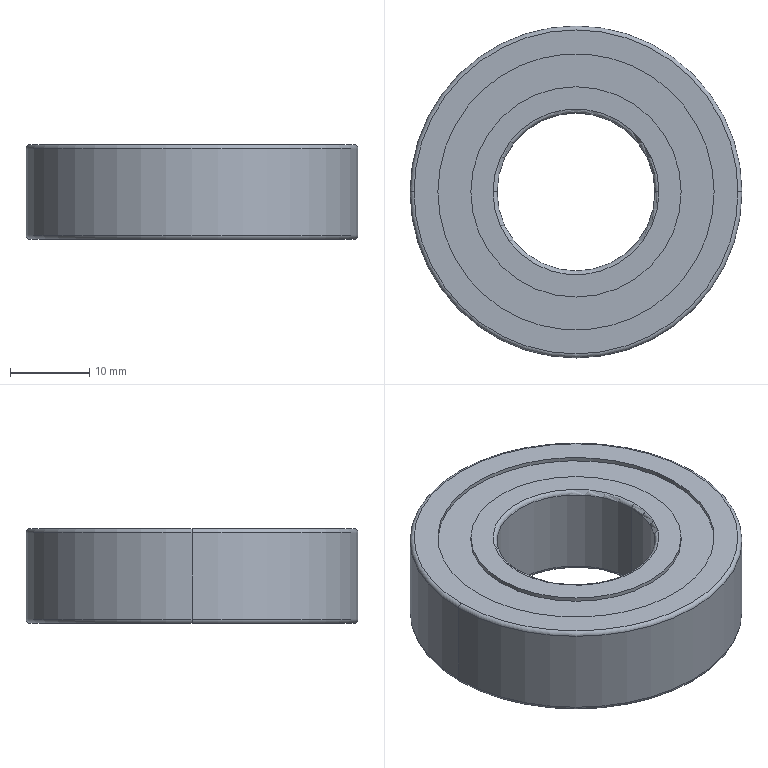Part | NX | features BREP 1 | 1 solid | 26 faces | box 42 x 42 x 12 mm | volume 12431 mm3 | cylinder 12 | torus 8 | plane 6 | commonest cylinder face diameters 26.623 x4 34.959 x4 20 x2 42 x2
STEP:
#1=CARTESIAN_POINT('',(13.311,0.,5.5));
#2=VERTEX_POINT('',#1);
#3=CARTESIAN_POINT('',(-13.311,0.,5.5));
#4=VERTEX_POINT('',#3);
#5=CARTESIAN_POINT('',(0.,0.,5.5));
#6=DIRECTION('',(0.,0.,-1.));
#7=DIRECTION('',(1.,0.,0.));
#8=AXIS2_PLACEMENT_3D('',#5,#6,#7);
#9=CIRCLE('',#8,13.311);
#10=EDGE_CURVE('',#2,#4,#9,.T.);
#11=ORIENTED_EDGE('',*,*,#10,.F.);
#12=CARTESIAN_POINT('',(13.311,0.,6.));
#13=VERTEX_POINT('',#12);
#14=CARTESIAN_POINT('',(13.311,0.,6.));
#15=DIRECTION('',(0.,0.,-1.));
#16=VECTOR('',#15,1000.);
#17=LINE('',#14,#16);
#18=EDGE_CURVE('',#13,#2,#17,.T.);
#19=ORIENTED_EDGE('',*,*,#18,.F.);
#20=CARTESIAN_POINT('',(-13.311,0.,6.));
#21=VERTEX_POINT('',#20);
#22=CARTESIAN_POINT('',(0.,0.,6.));
#23=DIRECTION('',(0.,0.,1.));
#24=DIRECTION('',(-1.,0.,0.));
#25=AXIS2_PLACEMENT_3D('',#22,#23,#24);
#26=CIRCLE('',#25,13.311);
#27=EDGE_CURVE('',#21,#13,#26,.T.);
#28=ORIENTED_EDGE('',*,*,#27,.F.);
#29=CARTESIAN_POINT('',(-13.311,0.,6.));
#30=DIRECTION('',(0.,0.,-1.));
#31=VECTOR('',#30,1000.);
#32=LINE('',#29,#31);
#33=EDGE_CURVE('',#21,#4,#32,.T.);
#34=ORIENTED_EDGE('',*,*,#33,.T.);
#35=EDGE_LOOP('',(#11,#19,#28,#34));
#36=FACE_BOUND('',#35,.T.);
#37=CARTESIAN_POINT('',(0.,0.,5.5));
#38=DIRECTION('',(0.,0.,1.));
#39=DIRECTION('',(-1.,0.,0.));
#40=AXIS2_PLACEMENT_3D('',#37,#38,#39);
#41=CYLINDRICAL_SURFACE('',#40,13.311);
#42=ADVANCED_FACE('',(#36),#41,.T.);
#43=ORIENTED_EDGE('',*,*,#33,.F.);
#44=CARTESIAN_POINT('',(0.,0.,6.));
#45=DIRECTION('',(0.,0.,1.));
#46=DIRECTION('',(1.,0.,0.));
#47=AXIS2_PLACEMENT_3D('',#44,#45,#46);
#48=CIRCLE('',#47,13.311);
#49=EDGE_CURVE('',#13,#21,#48,.T.);
#50=ORIENTED_EDGE('',*,*,#49,.F.);
#51=ORIENTED_EDGE('',*,*,#18,.T.);
#52=CARTESIAN_POINT('',(0.,0.,5.5));
#53=DIRECTION('',(0.,0.,-1.));
#54=DIRECTION('',(-1.,0.,0.));
#55=AXIS2_PLACEMENT_3D('',#52,#53,#54);
#56=CIRCLE('',#55,13.311);
#57=EDGE_CURVE('',#4,#2,#56,.T.);
#58=ORIENTED_EDGE('',*,*,#57,.F.);
#59=EDGE_LOOP('',(#43,#50,#51,#58));
#60=FACE_BOUND('',#59,.T.);
#61=CARTESIAN_POINT('',(0.,0.,5.5));
#62=DIRECTION('',(0.,0.,1.));
#63=DIRECTION('',(-1.,0.,0.));
#64=AXIS2_PLACEMENT_3D('',#61,#62,#63);
#65=CYLINDRICAL_SURFACE('',#64,13.311);
#66=ADVANCED_FACE('',(#60),#65,.T.);
#67=CARTESIAN_POINT('',(-17.479,0.,5.5));
#68=VERTEX_POINT('',#67);
#69=CARTESIAN_POINT('',(17.479,0.,5.5));
#70=VERTEX_POINT('',#69);
#71=CARTESIAN_POINT('',(0.,0.,5.5));
#72=DIRECTION('',(0.,0.,1.));
#73=DIRECTION('',(-1.,0.,0.));
#74=AXIS2_PLACEMENT_3D('',#71,#72,#73);
#75=CIRCLE('',#74,17.479);
#76=EDGE_CURVE('',#68,#70,#75,.T.);
#77=ORIENTED_EDGE('',*,*,#76,.T.);
#78=CARTESIAN_POINT('',(0.,0.,5.5));
#79=DIRECTION('',(0.,0.,1.));
#80=DIRECTION('',(1.,0.,0.));
#81=AXIS2_PLACEMENT_3D('',#78,#79,#80);
#82=CIRCLE('',#81,17.479);
#83=EDGE_CURVE('',#70,#68,#82,.T.);
#84=ORIENTED_EDGE('',*,*,#83,.T.);
#85=EDGE_LOOP('',(#77,#84));
#86=FACE_BOUND('',#85,.T.);
#87=ORIENTED_EDGE('',*,*,#10,.T.);
#88=ORIENTED_EDGE('',*,*,#57,.T.);
#89=EDGE_LOOP('',(#87,#88));
#90=FACE_BOUND('',#89,.T.);
#91=CARTESIAN_POINT('',(0.,0.,5.5));
#92=DIRECTION('',(0.,0.,1.));
#93=DIRECTION('',(-1.,0.,0.));
#94=AXIS2_PLACEMENT_3D('',#91,#92,#93);
#95=PLANE('',#94);
#96=ADVANCED_FACE('',(#86,#90),#95,.T.);
#97=ORIENTED_EDGE('',*,*,#83,.F.);
#98=CARTESIAN_POINT('',(17.479,0.,6.));
#99=VERTEX_POINT('',#98);
#100=CARTESIAN_POINT('',(17.479,0.,6.));
#101=DIRECTION('',(0.,0.,-1.));
#102=VECTOR('',#101,1000.);
#103=LINE('',#100,#102);
#104=EDGE_CURVE('',#99,#70,#103,.T.);
#105=ORIENTED_EDGE('',*,*,#104,.F.);
#106=CARTESIAN_POINT('',(-17.479,0.,6.));
#107=VERTEX_POINT('',#106);
#108=CARTESIAN_POINT('',(0.,0.,6.));
#109=DIRECTION('',(0.,0.,-1.));
#110=DIRECTION('',(-1.,0.,0.));
#111=AXIS2_PLACEMENT_3D('',#108,#109,#110);
#112=CIRCLE('',#111,17.479);
#113=EDGE_CURVE('',#107,#99,#112,.T.);
#114=ORIENTED_EDGE('',*,*,#113,.F.);
#115=CARTESIAN_POINT('',(-17.479,0.,6.));
#116=DIRECTION('',(0.,0.,-1.));
#117=VECTOR('',#116,1000.);
#118=LINE('',#115,#117);
#119=EDGE_CURVE('',#107,#68,#118,.T.);
#120=ORIENTED_EDGE('',*,*,#119,.T.);
#121=EDGE_LOOP('',(#97,#105,#114,#120));
#122=FACE_BOUND('',#121,.T.);
#123=CARTESIAN_POINT('',(0.,0.,5.5));
#124=DIRECTION('',(0.,0.,1.));
#125=DIRECTION('',(-1.,0.,0.));
#126=AXIS2_PLACEMENT_3D('',#123,#124,#125);
#127=CYLINDRICAL_SURFACE('',#126,17.479);
#128=ADVANCED_FACE('',(#122),#127,.F.);
#129=ORIENTED_EDGE('',*,*,#119,.F.);
#130=CARTESIAN_POINT('',(0.,0.,6.));
#131=DIRECTION('',(0.,0.,-1.));
#132=DIRECTION('',(1.,0.,0.));
#133=AXIS2_PLACEMENT_3D('',#130,#131,#132);
#134=CIRCLE('',#133,17.479);
#135=EDGE_CURVE('',#99,#107,#134,.T.);
#136=ORIENTED_EDGE('',*,*,#135,.F.);
#137=ORIENTED_EDGE('',*,*,#104,.T.);
#138=ORIENTED_EDGE('',*,*,#76,.F.);
#139=EDGE_LOOP('',(#129,#136,#137,#138));
#140=FACE_BOUND('',#139,.T.);
#141=CARTESIAN_POINT('',(0.,0.,5.5));
#142=DIRECTION('',(0.,0.,1.));
#143=DIRECTION('',(-1.,0.,0.));
#144=AXIS2_PLACEMENT_3D('',#141,#142,#143);
#145=CYLINDRICAL_SURFACE('',#144,17.479);
#146=ADVANCED_FACE('',(#140),#145,.F.);
#147=CARTESIAN_POINT('',(-20.5,0.,6.));
#148=VERTEX_POINT('',#147);
#149=CARTESIAN_POINT('',(20.5,0.,6.));
#150=VERTEX_POINT('',#149);
#151=CARTESIAN_POINT('',(0.,0.,6.));
#152=DIRECTION('',(0.,0.,1.));
#153=DIRECTION('',(-1.,0.,0.));
#154=AXIS2_PLACEMENT_3D('',#151,#152,#153);
#155=CIRCLE('',#154,20.5);
#156=EDGE_CURVE('',#148,#150,#155,.T.);
#157=ORIENTED_EDGE('',*,*,#156,.T.);
#158=CARTESIAN_POINT('',(0.,0.,6.));
#159=DIRECTION('',(0.,0.,1.));
#160=DIRECTION('',(1.,0.,0.));
#161=AXIS2_PLACEMENT_3D('',#158,#159,#160);
#162=CIRCLE('',#161,20.5);
#163=EDGE_CURVE('',#150,#148,#162,.T.);
#164=ORIENTED_EDGE('',*,*,#163,.T.);
#165=EDGE_LOOP('',(#157,#164));
#166=FACE_BOUND('',#165,.T.);
#167=ORIENTED_EDGE('',*,*,#135,.T.);
#168=ORIENTED_EDGE('',*,*,#113,.T.);
#169=EDGE_LOOP('',(#167,#168));
#170=FACE_BOUND('',#169,.T.);
#171=CARTESIAN_POINT('',(0.,0.,6.));
#172=DIRECTION('',(0.,0.,1.));
#173=DIRECTION('',(-1.,0.,0.));
#174=AXIS2_PLACEMENT_3D('',#171,#172,#173);
#175=PLANE('',#174);
#176=ADVANCED_FACE('',(#166,#170),#175,.T.);
#177=CARTESIAN_POINT('',(-21.,0.,5.5));
#178=VERTEX_POINT('',#177);
#179=CARTESIAN_POINT('',(-20.5,0.,5.5));
#180=DIRECTION('',(0.,-1.,0.));
#181=DIRECTION('',(0.,0.,1.));
#182=AXIS2_PLACEMENT_3D('',#179,#180,#181);
#183=CIRCLE('',#182,0.5);
#184=EDGE_CURVE('',#178,#148,#183,.F.);
#185=ORIENTED_EDGE('',*,*,#184,.T.);
#186=ORIENTED_EDGE('',*,*,#163,.F.);
#187=CARTESIAN_POINT('',(21.,0.,5.5));
#188=VERTEX_POINT('',#187);
#189=CARTESIAN_POINT('',(20.5,0.,5.5));
#190=DIRECTION('',(0.,1.,0.));
#191=DIRECTION('',(0.,0.,1.));
#192=AXIS2_PLACEMENT_3D('',#189,#190,#191);
#193=CIRCLE('',#192,0.5);
#194=EDGE_CURVE('',#188,#150,#193,.F.);
#195=ORIENTED_EDGE('',*,*,#194,.F.);
#196=CARTESIAN_POINT('',(0.,0.,5.5));
#197=DIRECTION('',(0.,0.,1.));
#198=DIRECTION('',(1.,0.,0.));
#199=AXIS2_PLACEMENT_3D('',#196,#197,#198);
#200=CIRCLE('',#199,21.);
#201=EDGE_CURVE('',#188,#178,#200,.T.);
#202=ORIENTED_EDGE('',*,*,#201,.T.);
#203=EDGE_LOOP('',(#185,#186,#195,#202));
#204=FACE_BOUND('',#203,.T.);
#205=CARTESIAN_POINT('',(0.,0.,5.5));
#206=DIRECTION('',(0.,0.,1.));
#207=DIRECTION('',(-1.,0.,0.));
#208=AXIS2_PLACEMENT_3D('',#205,#206,#207);
#209=TOROIDAL_SURFACE('',#208,20.5,0.5);
#210=ADVANCED_FACE('',(#204),#209,.T.);
#211=CARTESIAN_POINT('',(21.,0.,-5.5));
#212=VERTEX_POINT('',#211);
#213=CARTESIAN_POINT('',(21.,0.,-5.5));
#214=DIRECTION('',(0.,0.,1.));
#215=VECTOR('',#214,1000.);
#216=LINE('',#213,#215);
#217=EDGE_CURVE('',#212,#188,#216,.T.);
#218=ORIENTED_EDGE('',*,*,#217,.F.);
#219=CARTESIAN_POINT('',(-21.,0.,-5.5));
#220=VERTEX_POINT('',#219);
#221=CARTESIAN_POINT('',(0.,0.,-5.5));
#222=DIRECTION('',(0.,0.,-1.));
#223=DIRECTION('',(-1.,0.,0.));
#224=AXIS2_PLACEMENT_3D('',#221,#222,#223);
#225=CIRCLE('',#224,21.);
#226=EDGE_CURVE('',#220,#212,#225,.T.);
#227=ORIENTED_EDGE('',*,*,#226,.F.);
#228=CARTESIAN_POINT('',(-21.,0.,-5.5));
#229=DIRECTION('',(0.,0.,1.));
#230=VECTOR('',#229,1000.);
#231=LINE('',#228,#230);
#232=EDGE_CURVE('',#220,#178,#231,.T.);
#233=ORIENTED_EDGE('',*,*,#232,.T.);
#234=ORIENTED_EDGE('',*,*,#201,.F.);
#235=EDGE_LOOP('',(#218,#227,#233,#234));
#236=FACE_BOUND('',#235,.T.);
#237=CARTESIAN_POINT('',(0.,0.,6.));
#238=DIRECTION('',(0.,0.,-1.));
#239=DIRECTION('',(1.,0.,0.));
#240=AXIS2_PLACEMENT_3D('',#237,#238,#239);
#241=CYLINDRICAL_SURFACE('',#240,21.);
#242=ADVANCED_FACE('',(#236),#241,.T.);
#243=CARTESIAN_POINT('',(0.,0.,5.5));
#244=DIRECTION('',(0.,0.,1.));
#245=DIRECTION('',(-1.,0.,0.));
#246=AXIS2_PLACEMENT_3D('',#243,#244,#245);
#247=CIRCLE('',#246,21.);
#248=EDGE_CURVE('',#178,#188,#247,.T.);
#249=ORIENTED_EDGE('',*,*,#248,.F.);
#250=ORIENTED_EDGE('',*,*,#232,.F.);
#251=CARTESIAN_POINT('',(0.,0.,-5.5));
#252=DIRECTION('',(0.,0.,-1.));
#253=DIRECTION('',(1.,0.,0.));
#254=AXIS2_PLACEMENT_3D('',#251,#252,#253);
#255=CIRCLE('',#254,21.);
#256=EDGE_CURVE('',#212,#220,#255,.T.);
#257=ORIENTED_EDGE('',*,*,#256,.F.);
#258=ORIENTED_EDGE('',*,*,#217,.T.);
#259=EDGE_LOOP('',(#249,#250,#257,#258));
#260=FACE_BOUND('',#259,.T.);
#261=CARTESIAN_POINT('',(0.,0.,6.));
#262=DIRECTION('',(0.,0.,-1.));
#263=DIRECTION('',(1.,0.,0.));
#264=AXIS2_PLACEMENT_3D('',#261,#262,#263);
#265=CYLINDRICAL_SURFACE('',#264,21.);
#266=ADVANCED_FACE('',(#260),#265,.T.);
#267=CARTESIAN_POINT('',(20.5,0.,-6.));
#268=VERTEX_POINT('',#267);
#269=CARTESIAN_POINT('',(-20.5,0.,-6.));
#270=VERTEX_POINT('',#269);
#271=CARTESIAN_POINT('',(0.,0.,-6.));
#272=DIRECTION('',(0.,0.,-1.));
#273=DIRECTION('',(1.,0.,0.));
#274=AXIS2_PLACEMENT_3D('',#271,#272,#273);
#275=CIRCLE('',#274,20.5);
#276=EDGE_CURVE('',#268,#270,#275,.T.);
#277=ORIENTED_EDGE('',*,*,#276,.F.);
#278=CARTESIAN_POINT('',(20.5,0.,-5.5));
#279=DIRECTION('',(0.,1.,0.));
#280=DIRECTION('',(1.,0.,0.));
#281=AXIS2_PLACEMENT_3D('',#278,#279,#280);
#282=CIRCLE('',#281,0.5);
#283=EDGE_CURVE('',#212,#268,#282,.T.);
#284=ORIENTED_EDGE('',*,*,#283,.F.);
#285=ORIENTED_EDGE('',*,*,#256,.T.);
#286=CARTESIAN_POINT('',(-20.5,0.,-5.5));
#287=DIRECTION('',(0.,-1.,0.));
#288=DIRECTION('',(-1.,0.,0.));
#289=AXIS2_PLACEMENT_3D('',#286,#287,#288);
#290=CIRCLE('',#289,0.5);
#291=EDGE_CURVE('',#220,#270,#290,.T.);
#292=ORIENTED_EDGE('',*,*,#291,.T.);
#293=EDGE_LOOP('',(#277,#284,#285,#292));
#294=FACE_BOUND('',#293,.T.);
#295=CARTESIAN_POINT('',(0.,0.,-5.5));
#296=DIRECTION('',(0.,0.,1.));
#297=DIRECTION('',(-1.,0.,0.));
#298=AXIS2_PLACEMENT_3D('',#295,#296,#297);
#299=TOROIDAL_SURFACE('',#298,20.5,0.5);
#300=ADVANCED_FACE('',(#294),#299,.T.);
#301=ORIENTED_EDGE('',*,*,#291,.F.);
#302=ORIENTED_EDGE('',*,*,#226,.T.);
#303=ORIENTED_EDGE('',*,*,#283,.T.);
#304=CARTESIAN_POINT('',(0.,0.,-6.));
#305=DIRECTION('',(0.,0.,-1.));
#306=DIRECTION('',(-1.,0.,0.));
#307=AXIS2_PLACEMENT_3D('',#304,#305,#306);
#308=CIRCLE('',#307,20.5);
#309=EDGE_CURVE('',#270,#268,#308,.T.);
#310=ORIENTED_EDGE('',*,*,#309,.F.);
#311=EDGE_LOOP('',(#301,#302,#303,#310));
#312=FACE_BOUND('',#311,.T.);
#313=CARTESIAN_POINT('',(0.,0.,-5.5));
#314=DIRECTION('',(0.,0.,1.));
#315=DIRECTION('',(-1.,0.,0.));
#316=AXIS2_PLACEMENT_3D('',#313,#314,#315);
#317=TOROIDAL_SURFACE('',#316,20.5,0.5);
#318=ADVANCED_FACE('',(#312),#317,.T.);
#319=ORIENTED_EDGE('',*,*,#309,.T.);
#320=ORIENTED_EDGE('',*,*,#276,.T.);
#321=EDGE_LOOP('',(#319,#320));
#322=FACE_BOUND('',#321,.T.);
#323=CARTESIAN_POINT('',(17.479,0.,-6.));
#324=VERTEX_POINT('',#323);
#325=CARTESIAN_POINT('',(-17.479,0.,-6.));
#326=VERTEX_POINT('',#325);
#327=CARTESIAN_POINT('',(0.,0.,-6.));
#328=DIRECTION('',(0.,0.,1.));
#329=DIRECTION('',(1.,0.,0.));
#330=AXIS2_PLACEMENT_3D('',#327,#328,#329);
#331=CIRCLE('',#330,17.479);
#332=EDGE_CURVE('',#324,#326,#331,.T.);
#333=ORIENTED_EDGE('',*,*,#332,.T.);
#334=CARTESIAN_POINT('',(0.,0.,-6.));
#335=DIRECTION('',(0.,0.,1.));
#336=DIRECTION('',(-1.,0.,0.));
#337=AXIS2_PLACEMENT_3D('',#334,#335,#336);
#338=CIRCLE('',#337,17.479);
#339=EDGE_CURVE('',#326,#324,#338,.T.);
#340=ORIENTED_EDGE('',*,*,#339,.T.);
#341=EDGE_LOOP('',(#333,#340));
#342=FACE_BOUND('',#341,.T.);
#343=CARTESIAN_POINT('',(0.,0.,-6.));
#344=DIRECTION('',(0.,0.,1.));
#345=DIRECTION('',(-1.,0.,0.));
#346=AXIS2_PLACEMENT_3D('',#343,#344,#345);
#347=PLANE('',#346);
#348=ADVANCED_FACE('',(#322,#342),#347,.F.);
#349=CARTESIAN_POINT('',(17.479,0.,-5.5));
#350=VERTEX_POINT('',#349);
#351=CARTESIAN_POINT('',(17.479,0.,-6.));
#352=DIRECTION('',(0.,0.,1.));
#353=VECTOR('',#352,1000.);
#354=LINE('',#351,#353);
#355=EDGE_CURVE('',#324,#350,#354,.T.);
#356=ORIENTED_EDGE('',*,*,#355,.F.);
#357=ORIENTED_EDGE('',*,*,#339,.F.);
#358=CARTESIAN_POINT('',(-17.479,0.,-5.5));
#359=VERTEX_POINT('',#358);
#360=CARTESIAN_POINT('',(-17.479,0.,-6.));
#361=DIRECTION('',(0.,0.,1.));
#362=VECTOR('',#361,1000.);
#363=LINE('',#360,#362);
#364=EDGE_CURVE('',#326,#359,#363,.T.);
#365=ORIENTED_EDGE('',*,*,#364,.T.);
#366=CARTESIAN_POINT('',(0.,0.,-5.5));
#367=DIRECTION('',(0.,0.,-1.));
#368=DIRECTION('',(1.,0.,0.));
#369=AXIS2_PLACEMENT_3D('',#366,#367,#368);
#370=CIRCLE('',#369,17.479);
#371=EDGE_CURVE('',#350,#359,#370,.T.);
#372=ORIENTED_EDGE('',*,*,#371,.F.);
#373=EDGE_LOOP('',(#356,#357,#365,#372));
#374=FACE_BOUND('',#373,.T.);
#375=CARTESIAN_POINT('',(0.,0.,-5.5));
#376=DIRECTION('',(0.,0.,-1.));
#377=DIRECTION('',(1.,0.,0.));
#378=AXIS2_PLACEMENT_3D('',#375,#376,#377);
#379=CYLINDRICAL_SURFACE('',#378,17.479);
#380=ADVANCED_FACE('',(#374),#379,.F.);
#381=CARTESIAN_POINT('',(0.,0.,-5.5));
#382=DIRECTION('',(0.,0.,-1.));
#383=DIRECTION('',(-1.,0.,0.));
#384=AXIS2_PLACEMENT_3D('',#381,#382,#383);
#385=CIRCLE('',#384,17.479);
#386=EDGE_CURVE('',#359,#350,#385,.T.);
#387=ORIENTED_EDGE('',*,*,#386,.T.);
#388=ORIENTED_EDGE('',*,*,#371,.T.);
#389=EDGE_LOOP('',(#387,#388));
#390=FACE_BOUND('',#389,.T.);
#391=CARTESIAN_POINT('',(13.311,0.,-5.5));
#392=VERTEX_POINT('',#391);
#393=CARTESIAN_POINT('',(-13.311,0.,-5.5));
#394=VERTEX_POINT('',#393);
#395=CARTESIAN_POINT('',(0.,0.,-5.5));
#396=DIRECTION('',(0.,0.,1.));
#397=DIRECTION('',(1.,0.,0.));
#398=AXIS2_PLACEMENT_3D('',#395,#396,#397);
#399=CIRCLE('',#398,13.311);
#400=EDGE_CURVE('',#392,#394,#399,.T.);
#401=ORIENTED_EDGE('',*,*,#400,.T.);
#402=CARTESIAN_POINT('',(0.,0.,-5.5));
#403=DIRECTION('',(0.,0.,1.));
#404=DIRECTION('',(-1.,0.,0.));
#405=AXIS2_PLACEMENT_3D('',#402,#403,#404);
#406=CIRCLE('',#405,13.311);
#407=EDGE_CURVE('',#394,#392,#406,.T.);
#408=ORIENTED_EDGE('',*,*,#407,.T.);
#409=EDGE_LOOP('',(#401,#408));
#410=FACE_BOUND('',#409,.T.);
#411=CARTESIAN_POINT('',(0.,0.,-5.5));
#412=DIRECTION('',(0.,0.,-1.));
#413=DIRECTION('',(-1.,0.,0.));
#414=AXIS2_PLACEMENT_3D('',#411,#412,#413);
#415=PLANE('',#414);
#416=ADVANCED_FACE('',(#390,#410),#415,.T.);
#417=ORIENTED_EDGE('',*,*,#386,.F.);
#418=ORIENTED_EDGE('',*,*,#364,.F.);
#419=ORIENTED_EDGE('',*,*,#332,.F.);
#420=ORIENTED_EDGE('',*,*,#355,.T.);
#421=EDGE_LOOP('',(#417,#418,#419,#420));
#422=FACE_BOUND('',#421,.T.);
#423=CARTESIAN_POINT('',(0.,0.,-5.5));
#424=DIRECTION('',(0.,0.,-1.));
#425=DIRECTION('',(1.,0.,0.));
#426=AXIS2_PLACEMENT_3D('',#423,#424,#425);
#427=CYLINDRICAL_SURFACE('',#426,17.479);
#428=ADVANCED_FACE('',(#422),#427,.F.);
#429=ORIENTED_EDGE('',*,*,#407,.F.);
#430=CARTESIAN_POINT('',(-13.311,0.,-6.));
#431=VERTEX_POINT('',#430);
#432=CARTESIAN_POINT('',(-13.311,0.,-6.));
#433=DIRECTION('',(0.,0.,1.));
#434=VECTOR('',#433,1000.);
#435=LINE('',#432,#434);
#436=EDGE_CURVE('',#394,#431,#435,.F.);
#437=ORIENTED_EDGE('',*,*,#436,.T.);
#438=CARTESIAN_POINT('',(13.311,0.,-6.));
#439=VERTEX_POINT('',#438);
#440=CARTESIAN_POINT('',(0.,0.,-6.));
#441=DIRECTION('',(0.,0.,-1.));
#442=DIRECTION('',(1.,0.,0.));
#443=AXIS2_PLACEMENT_3D('',#440,#441,#442);
#444=CIRCLE('',#443,13.311);
#445=EDGE_CURVE('',#439,#431,#444,.T.);
#446=ORIENTED_EDGE('',*,*,#445,.F.);
#447=CARTESIAN_POINT('',(13.311,0.,-6.));
#448=DIRECTION('',(0.,0.,1.));
#449=VECTOR('',#448,1000.);
#450=LINE('',#447,#449);
#451=EDGE_CURVE('',#392,#439,#450,.F.);
#452=ORIENTED_EDGE('',*,*,#451,.F.);
#453=EDGE_LOOP('',(#429,#437,#446,#452));
#454=FACE_BOUND('',#453,.T.);
#455=CARTESIAN_POINT('',(0.,0.,-5.5));
#456=DIRECTION('',(0.,0.,-1.));
#457=DIRECTION('',(1.,0.,0.));
#458=AXIS2_PLACEMENT_3D('',#455,#456,#457);
#459=CYLINDRICAL_SURFACE('',#458,13.311);
#460=ADVANCED_FACE('',(#454),#459,.T.);
#461=ORIENTED_EDGE('',*,*,#451,.T.);
#462=CARTESIAN_POINT('',(0.,0.,-6.));
#463=DIRECTION('',(0.,0.,-1.));
#464=DIRECTION('',(-1.,0.,0.));
#465=AXIS2_PLACEMENT_3D('',#462,#463,#464);
#466=CIRCLE('',#465,13.311);
#467=EDGE_CURVE('',#431,#439,#466,.T.);
#468=ORIENTED_EDGE('',*,*,#467,.F.);
#469=ORIENTED_EDGE('',*,*,#436,.F.);
#470=ORIENTED_EDGE('',*,*,#400,.F.);
#471=EDGE_LOOP('',(#461,#468,#469,#470));
#472=FACE_BOUND('',#471,.T.);
#473=CARTESIAN_POINT('',(0.,0.,-5.5));
#474=DIRECTION('',(0.,0.,-1.));
#475=DIRECTION('',(1.,0.,0.));
#476=AXIS2_PLACEMENT_3D('',#473,#474,#475);
#477=CYLINDRICAL_SURFACE('',#476,13.311);
#478=ADVANCED_FACE('',(#472),#477,.T.);
#479=ORIENTED_EDGE('',*,*,#467,.T.);
#480=ORIENTED_EDGE('',*,*,#445,.T.);
#481=EDGE_LOOP('',(#479,#480));
#482=FACE_BOUND('',#481,.T.);
#483=CARTESIAN_POINT('',(-10.5,0.,-6.));
#484=VERTEX_POINT('',#483);
#485=CARTESIAN_POINT('',(10.5,0.,-6.));
#486=VERTEX_POINT('',#485);
#487=CARTESIAN_POINT('',(0.,0.,-6.));
#488=DIRECTION('',(0.,0.,1.));
#489=DIRECTION('',(-1.,0.,0.));
#490=AXIS2_PLACEMENT_3D('',#487,#488,#489);
#491=CIRCLE('',#490,10.5);
#492=EDGE_CURVE('',#484,#486,#491,.T.);
#493=ORIENTED_EDGE('',*,*,#492,.T.);
#494=CARTESIAN_POINT('',(0.,0.,-6.));
#495=DIRECTION('',(0.,0.,1.));
#496=DIRECTION('',(1.,0.,0.));
#497=AXIS2_PLACEMENT_3D('',#494,#495,#496);
#498=CIRCLE('',#497,10.5);
#499=EDGE_CURVE('',#486,#484,#498,.T.);
#500=ORIENTED_EDGE('',*,*,#499,.T.);
#501=EDGE_LOOP('',(#493,#500));
#502=FACE_BOUND('',#501,.T.);
#503=CARTESIAN_POINT('',(0.,0.,-6.));
#504=DIRECTION('',(0.,0.,1.));
#505=DIRECTION('',(-1.,0.,0.));
#506=AXIS2_PLACEMENT_3D('',#503,#504,#505);
#507=PLANE('',#506);
#508=ADVANCED_FACE('',(#482,#502),#507,.F.);
#509=CARTESIAN_POINT('',(-10.,0.,-5.5));
#510=VERTEX_POINT('',#509);
#511=CARTESIAN_POINT('',(-10.5,0.,-5.5));
#512=DIRECTION('',(0.,-1.,0.));
#513=DIRECTION('',(0.,0.,-1.));
#514=AXIS2_PLACEMENT_3D('',#511,#512,#513);
#515=CIRCLE('',#514,0.5);
#516=EDGE_CURVE('',#510,#484,#515,.F.);
#517=ORIENTED_EDGE('',*,*,#516,.T.);
#518=ORIENTED_EDGE('',*,*,#499,.F.);
#519=CARTESIAN_POINT('',(10.,0.,-5.5));
#520=VERTEX_POINT('',#519);
#521=CARTESIAN_POINT('',(10.5,0.,-5.5));
#522=DIRECTION('',(0.,1.,0.));
#523=DIRECTION('',(0.,0.,-1.));
#524=AXIS2_PLACEMENT_3D('',#521,#522,#523);
#525=CIRCLE('',#524,0.5);
#526=EDGE_CURVE('',#520,#486,#525,.F.);
#527=ORIENTED_EDGE('',*,*,#526,.F.);
#528=CARTESIAN_POINT('',(0.,0.,-5.5));
#529=DIRECTION('',(0.,0.,1.));
#530=DIRECTION('',(1.,0.,0.));
#531=AXIS2_PLACEMENT_3D('',#528,#529,#530);
#532=CIRCLE('',#531,10.);
#533=EDGE_CURVE('',#520,#510,#532,.T.);
#534=ORIENTED_EDGE('',*,*,#533,.T.);
#535=EDGE_LOOP('',(#517,#518,#527,#534));
#536=FACE_BOUND('',#535,.T.);
#537=CARTESIAN_POINT('',(0.,0.,-5.5));
#538=DIRECTION('',(0.,0.,1.));
#539=DIRECTION('',(-1.,0.,0.));
#540=AXIS2_PLACEMENT_3D('',#537,#538,#539);
#541=TOROIDAL_SURFACE('',#540,10.5,0.5);
#542=ADVANCED_FACE('',(#536),#541,.T.);
#543=CARTESIAN_POINT('',(-10.,0.,5.5));
#544=VERTEX_POINT('',#543);
#545=CARTESIAN_POINT('',(10.,0.,5.5));
#546=VERTEX_POINT('',#545);
#547=CARTESIAN_POINT('',(0.,0.,5.5));
#548=DIRECTION('',(0.,0.,-1.));
#549=DIRECTION('',(-1.,0.,0.));
#550=AXIS2_PLACEMENT_3D('',#547,#548,#549);
#551=CIRCLE('',#550,10.);
#552=EDGE_CURVE('',#544,#546,#551,.T.);
#553=ORIENTED_EDGE('',*,*,#552,.F.);
#554=CARTESIAN_POINT('',(-10.,0.,-5.5));
#555=DIRECTION('',(0.,0.,1.));
#556=VECTOR('',#555,1000.);
#557=LINE('',#554,#556);
#558=EDGE_CURVE('',#544,#510,#557,.F.);
#559=ORIENTED_EDGE('',*,*,#558,.T.);
#560=ORIENTED_EDGE('',*,*,#533,.F.);
#561=CARTESIAN_POINT('',(10.,0.,-5.5));
#562=DIRECTION('',(0.,0.,1.));
#563=VECTOR('',#562,1000.);
#564=LINE('',#561,#563);
#565=EDGE_CURVE('',#546,#520,#564,.F.);
#566=ORIENTED_EDGE('',*,*,#565,.F.);
#567=EDGE_LOOP('',(#553,#559,#560,#566));
#568=FACE_BOUND('',#567,.T.);
#569=CARTESIAN_POINT('',(0.,0.,6.));
#570=DIRECTION('',(0.,0.,-1.));
#571=DIRECTION('',(1.,0.,0.));
#572=AXIS2_PLACEMENT_3D('',#569,#570,#571);
#573=CYLINDRICAL_SURFACE('',#572,10.);
#574=ADVANCED_FACE('',(#568),#573,.F.);
#575=ORIENTED_EDGE('',*,*,#565,.T.);
#576=CARTESIAN_POINT('',(0.,0.,-5.5));
#577=DIRECTION('',(0.,0.,1.));
#578=DIRECTION('',(-1.,0.,0.));
#579=AXIS2_PLACEMENT_3D('',#576,#577,#578);
#580=CIRCLE('',#579,10.);
#581=EDGE_CURVE('',#510,#520,#580,.T.);
#582=ORIENTED_EDGE('',*,*,#581,.F.);
#583=ORIENTED_EDGE('',*,*,#558,.F.);
#584=CARTESIAN_POINT('',(0.,0.,5.5));
#585=DIRECTION('',(0.,0.,-1.));
#586=DIRECTION('',(1.,0.,0.));
#587=AXIS2_PLACEMENT_3D('',#584,#585,#586);
#588=CIRCLE('',#587,10.);
#589=EDGE_CURVE('',#546,#544,#588,.T.);
#590=ORIENTED_EDGE('',*,*,#589,.F.);
#591=EDGE_LOOP('',(#575,#582,#583,#590));
#592=FACE_BOUND('',#591,.T.);
#593=CARTESIAN_POINT('',(0.,0.,6.));
#594=DIRECTION('',(0.,0.,-1.));
#595=DIRECTION('',(1.,0.,0.));
#596=AXIS2_PLACEMENT_3D('',#593,#594,#595);
#597=CYLINDRICAL_SURFACE('',#596,10.);
#598=ADVANCED_FACE('',(#592),#597,.F.);
#599=CARTESIAN_POINT('',(10.5,0.,6.));
#600=VERTEX_POINT('',#599);
#601=CARTESIAN_POINT('',(-10.5,0.,6.));
#602=VERTEX_POINT('',#601);
#603=CARTESIAN_POINT('',(0.,0.,6.));
#604=DIRECTION('',(0.,0.,-1.));
#605=DIRECTION('',(1.,0.,0.));
#606=AXIS2_PLACEMENT_3D('',#603,#604,#605);
#607=CIRCLE('',#606,10.5);
#608=EDGE_CURVE('',#600,#602,#607,.T.);
#609=ORIENTED_EDGE('',*,*,#608,.F.);
#610=CARTESIAN_POINT('',(10.5,0.,5.5));
#611=DIRECTION('',(0.,1.,0.));
#612=DIRECTION('',(-1.,0.,0.));
#613=AXIS2_PLACEMENT_3D('',#610,#611,#612);
#614=CIRCLE('',#613,0.5);
#615=EDGE_CURVE('',#546,#600,#614,.T.);
#616=ORIENTED_EDGE('',*,*,#615,.F.);
#617=ORIENTED_EDGE('',*,*,#589,.T.);
#618=CARTESIAN_POINT('',(-10.5,0.,5.5));
#619=DIRECTION('',(0.,-1.,0.));
#620=DIRECTION('',(1.,0.,0.));
#621=AXIS2_PLACEMENT_3D('',#618,#619,#620);
#622=CIRCLE('',#621,0.5);
#623=EDGE_CURVE('',#544,#602,#622,.T.);
#624=ORIENTED_EDGE('',*,*,#623,.T.);
#625=EDGE_LOOP('',(#609,#616,#617,#624));
#626=FACE_BOUND('',#625,.T.);
#627=CARTESIAN_POINT('',(0.,0.,5.5));
#628=DIRECTION('',(0.,0.,1.));
#629=DIRECTION('',(-1.,0.,0.));
#630=AXIS2_PLACEMENT_3D('',#627,#628,#629);
#631=TOROIDAL_SURFACE('',#630,10.5,0.5);
#632=ADVANCED_FACE('',(#626),#631,.T.);
#633=ORIENTED_EDGE('',*,*,#623,.F.);
#634=ORIENTED_EDGE('',*,*,#552,.T.);
#635=ORIENTED_EDGE('',*,*,#615,.T.);
#636=CARTESIAN_POINT('',(0.,0.,6.));
#637=DIRECTION('',(0.,0.,-1.));
#638=DIRECTION('',(-1.,0.,0.));
#639=AXIS2_PLACEMENT_3D('',#636,#637,#638);
#640=CIRCLE('',#639,10.5);
#641=EDGE_CURVE('',#602,#600,#640,.T.);
#642=ORIENTED_EDGE('',*,*,#641,.F.);
#643=EDGE_LOOP('',(#633,#634,#635,#642));
#644=FACE_BOUND('',#643,.T.);
#645=CARTESIAN_POINT('',(0.,0.,5.5));
#646=DIRECTION('',(0.,0.,1.));
#647=DIRECTION('',(-1.,0.,0.));
#648=AXIS2_PLACEMENT_3D('',#645,#646,#647);
#649=TOROIDAL_SURFACE('',#648,10.5,0.5);
#650=ADVANCED_FACE('',(#644),#649,.T.);
#651=ORIENTED_EDGE('',*,*,#27,.T.);
#652=ORIENTED_EDGE('',*,*,#49,.T.);
#653=EDGE_LOOP('',(#651,#652));
#654=FACE_BOUND('',#653,.T.);
#655=ORIENTED_EDGE('',*,*,#641,.T.);
#656=ORIENTED_EDGE('',*,*,#608,.T.);
#657=EDGE_LOOP('',(#655,#656));
#658=FACE_BOUND('',#657,.T.);
#659=CARTESIAN_POINT('',(0.,0.,6.));
#660=DIRECTION('',(0.,0.,1.));
#661=DIRECTION('',(-1.,0.,0.));
#662=AXIS2_PLACEMENT_3D('',#659,#660,#661);
#663=PLANE('',#662);
#664=ADVANCED_FACE('',(#654,#658),#663,.T.);
#665=ORIENTED_EDGE('',*,*,#581,.T.);
#666=ORIENTED_EDGE('',*,*,#526,.T.);
#667=ORIENTED_EDGE('',*,*,#492,.F.);
#668=ORIENTED_EDGE('',*,*,#516,.F.);
#669=EDGE_LOOP('',(#665,#666,#667,#668));
#670=FACE_BOUND('',#669,.T.);
#671=CARTESIAN_POINT('',(0.,0.,-5.5));
#672=DIRECTION('',(0.,0.,1.));
#673=DIRECTION('',(-1.,0.,0.));
#674=AXIS2_PLACEMENT_3D('',#671,#672,#673);
#675=TOROIDAL_SURFACE('',#674,10.5,0.5);
#676=ADVANCED_FACE('',(#670),#675,.T.);
#677=ORIENTED_EDGE('',*,*,#248,.T.);
#678=ORIENTED_EDGE('',*,*,#194,.T.);
#679=ORIENTED_EDGE('',*,*,#156,.F.);
#680=ORIENTED_EDGE('',*,*,#184,.F.);
#681=EDGE_LOOP('',(#677,#678,#679,#680));
#682=FACE_BOUND('',#681,.T.);
#683=CARTESIAN_POINT('',(0.,0.,5.5));
#684=DIRECTION('',(0.,0.,1.));
#685=DIRECTION('',(-1.,0.,0.));
#686=AXIS2_PLACEMENT_3D('',#683,#684,#685);
#687=TOROIDAL_SURFACE('',#686,20.5,0.5);
#688=ADVANCED_FACE('',(#682),#687,.T.);
#689=CLOSED_SHELL('',(#42,#66,#96,#128,#146,#176,#210,#242,#266,#300,#318,#348,#380,#416,#428,#460,#478,#508,#542,#574,#598,#632,#650,#664,#676,#688));
#690=MANIFOLD_SOLID_BREP('',#689);
#691=(LENGTH_UNIT()NAMED_UNIT(*)SI_UNIT(.MILLI.,.METRE.));
#692=UNCERTAINTY_MEASURE_WITH_UNIT(LENGTH_MEASURE(0.00001),#691,'','');
#693=(NAMED_UNIT(*)PLANE_ANGLE_UNIT()SI_UNIT($,.RADIAN.));
#694=(NAMED_UNIT(*)SI_UNIT($,.STERADIAN.)SOLID_ANGLE_UNIT());
#695=(GEOMETRIC_REPRESENTATION_CONTEXT(3)GLOBAL_UNCERTAINTY_ASSIGNED_CONTEXT((#692))GLOBAL_UNIT_ASSIGNED_CONTEXT((#691,#693,#694))REPRESENTATION_CONTEXT('',''));
#696=ADVANCED_BREP_SHAPE_REPRESENTATION('',(#690),#695);